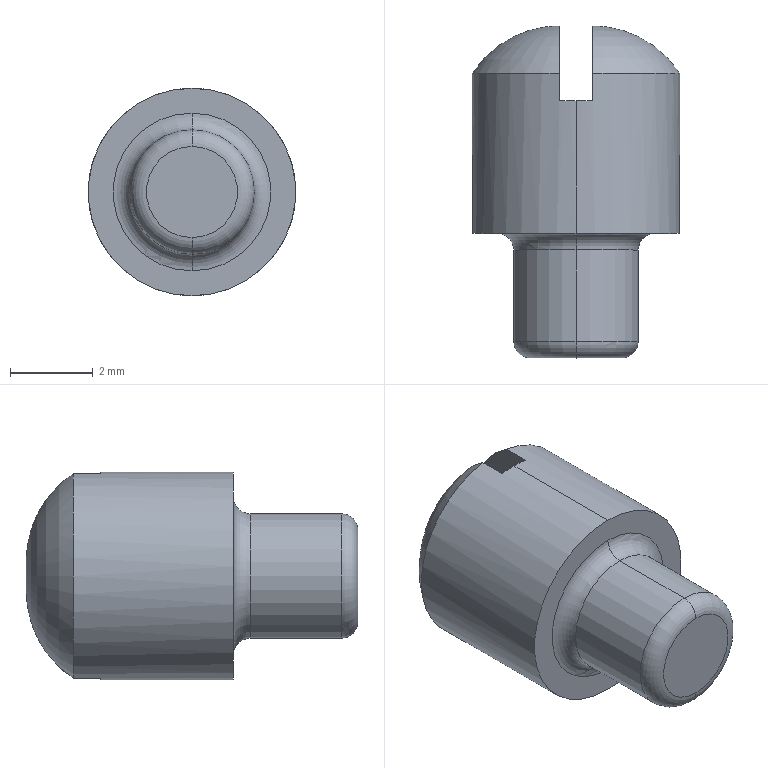Part | SolidWorks | features Fillet 2, ICE 1, Revolution 1 | 1 solid | 15 faces | box 5 x 8 x 5 mm | volume 104.473 mm3 | torus 6 | plane 5 | cylinder 4 | commonest cylinder face diameters 3 x2 5 x2
STEP:
#1=CARTESIAN_POINT('',(0.,0.4,1.5));
#2=VERTEX_POINT('',#1);
#3=CARTESIAN_POINT('',(0.,0.4,-1.5));
#4=VERTEX_POINT('',#3);
#5=CARTESIAN_POINT('',(0.,0.4,0.));
#6=DIRECTION('',(0.,1.,0.));
#7=DIRECTION('',(0.,0.,-1.));
#8=AXIS2_PLACEMENT_3D('',#5,#6,#7);
#9=CIRCLE('',#8,1.5);
#10=EDGE_CURVE('',#2,#4,#9,.T.);
#11=ORIENTED_EDGE('',*,*,#10,.F.);
#12=CARTESIAN_POINT('',(0.,0.,1.1));
#13=VERTEX_POINT('',#12);
#14=CARTESIAN_POINT('',(0.,0.4,1.1));
#15=DIRECTION('',(1.,0.,0.));
#16=DIRECTION('',(0.,0.,-1.));
#17=AXIS2_PLACEMENT_3D('',#14,#15,#16);
#18=CIRCLE('',#17,0.4);
#19=EDGE_CURVE('',#2,#13,#18,.T.);
#20=ORIENTED_EDGE('',*,*,#19,.T.);
#21=CARTESIAN_POINT('',(0.,0.,-1.1));
#22=VERTEX_POINT('',#21);
#23=CARTESIAN_POINT('',(0.,0.,0.));
#24=DIRECTION('',(0.,-1.,0.));
#25=DIRECTION('',(0.,0.,-1.));
#26=AXIS2_PLACEMENT_3D('',#23,#24,#25);
#27=CIRCLE('',#26,1.1);
#28=EDGE_CURVE('',#22,#13,#27,.T.);
#29=ORIENTED_EDGE('',*,*,#28,.F.);
#30=CARTESIAN_POINT('',(0.,0.4,-1.1));
#31=DIRECTION('',(-1.,0.,0.));
#32=DIRECTION('',(0.,0.,1.));
#33=AXIS2_PLACEMENT_3D('',#30,#31,#32);
#34=CIRCLE('',#33,0.4);
#35=EDGE_CURVE('',#4,#22,#34,.T.);
#36=ORIENTED_EDGE('',*,*,#35,.F.);
#37=EDGE_LOOP('',(#11,#20,#29,#36));
#38=FACE_OUTER_BOUND('',#37,.T.);
#39=CARTESIAN_POINT('',(0.,0.4,0.));
#40=DIRECTION('',(0.,-1.,0.));
#41=DIRECTION('',(0.,0.,-1.));
#42=AXIS2_PLACEMENT_3D('',#39,#40,#41);
#43=TOROIDAL_SURFACE('',#42,1.1,0.4);
#44=ADVANCED_FACE('',(#38),#43,.T.);
#45=CARTESIAN_POINT('',(0.,2.6,1.5));
#46=VERTEX_POINT('',#45);
#47=CARTESIAN_POINT('',(0.,2.6,-1.5));
#48=VERTEX_POINT('',#47);
#49=CARTESIAN_POINT('',(0.,2.6,0.));
#50=DIRECTION('',(0.,-1.,0.));
#51=DIRECTION('',(0.,0.,-1.));
#52=AXIS2_PLACEMENT_3D('',#49,#50,#51);
#53=CIRCLE('',#52,1.5);
#54=EDGE_CURVE('',#46,#48,#53,.T.);
#55=ORIENTED_EDGE('',*,*,#54,.F.);
#56=CARTESIAN_POINT('',(0.,3.,1.9));
#57=VERTEX_POINT('',#56);
#58=CARTESIAN_POINT('',(0.,2.6,1.9));
#59=DIRECTION('',(1.,0.,0.));
#60=DIRECTION('',(0.,0.,-1.));
#61=AXIS2_PLACEMENT_3D('',#58,#59,#60);
#62=CIRCLE('',#61,0.4);
#63=EDGE_CURVE('',#46,#57,#62,.T.);
#64=ORIENTED_EDGE('',*,*,#63,.T.);
#65=CARTESIAN_POINT('',(0.,3.,-1.9));
#66=VERTEX_POINT('',#65);
#67=CARTESIAN_POINT('',(0.,3.,0.));
#68=DIRECTION('',(0.,1.,0.));
#69=DIRECTION('',(0.,0.,-1.));
#70=AXIS2_PLACEMENT_3D('',#67,#68,#69);
#71=CIRCLE('',#70,1.9);
#72=EDGE_CURVE('',#66,#57,#71,.T.);
#73=ORIENTED_EDGE('',*,*,#72,.F.);
#74=CARTESIAN_POINT('',(0.,2.6,-1.9));
#75=DIRECTION('',(-1.,0.,0.));
#76=DIRECTION('',(0.,0.,1.));
#77=AXIS2_PLACEMENT_3D('',#74,#75,#76);
#78=CIRCLE('',#77,0.4);
#79=EDGE_CURVE('',#48,#66,#78,.T.);
#80=ORIENTED_EDGE('',*,*,#79,.F.);
#81=EDGE_LOOP('',(#55,#64,#73,#80));
#82=FACE_OUTER_BOUND('',#81,.T.);
#83=CARTESIAN_POINT('',(0.,2.6,0.));
#84=DIRECTION('',(0.,-1.,0.));
#85=DIRECTION('',(0.,0.,-1.));
#86=AXIS2_PLACEMENT_3D('',#83,#84,#85);
#87=TOROIDAL_SURFACE('',#86,1.9,0.4);
#88=ADVANCED_FACE('',(#82),#87,.F.);
#89=ORIENTED_EDGE('',*,*,#10,.T.);
#90=CARTESIAN_POINT('',(0.,5.056,-1.5));
#91=DIRECTION('',(0.,1.,0.));
#92=VECTOR('',#91,1000.);
#93=LINE('',#90,#92);
#94=EDGE_CURVE('',#4,#48,#93,.T.);
#95=ORIENTED_EDGE('',*,*,#94,.T.);
#96=CARTESIAN_POINT('',(0.,2.6,0.));
#97=DIRECTION('',(0.,-1.,0.));
#98=DIRECTION('',(0.,0.,-1.));
#99=AXIS2_PLACEMENT_3D('',#96,#97,#98);
#100=CIRCLE('',#99,1.5);
#101=EDGE_CURVE('',#48,#46,#100,.T.);
#102=ORIENTED_EDGE('',*,*,#101,.T.);
#103=CARTESIAN_POINT('',(0.,5.056,1.5));
#104=DIRECTION('',(0.,1.,0.));
#105=VECTOR('',#104,1000.);
#106=LINE('',#103,#105);
#107=EDGE_CURVE('',#2,#46,#106,.T.);
#108=ORIENTED_EDGE('',*,*,#107,.F.);
#109=EDGE_LOOP('',(#89,#95,#102,#108));
#110=FACE_OUTER_BOUND('',#109,.T.);
#111=CARTESIAN_POINT('',(0.,5.056,0.));
#112=DIRECTION('',(0.,1.,0.));
#113=DIRECTION('',(0.,0.,1.));
#114=AXIS2_PLACEMENT_3D('',#111,#112,#113);
#115=CYLINDRICAL_SURFACE('',#114,1.5);
#116=ADVANCED_FACE('',(#110),#115,.T.);
#117=CARTESIAN_POINT('',(0.,3.,2.5));
#118=VERTEX_POINT('',#117);
#119=CARTESIAN_POINT('',(0.,3.,-2.5));
#120=VERTEX_POINT('',#119);
#121=CARTESIAN_POINT('',(0.,3.,0.));
#122=DIRECTION('',(0.,1.,0.));
#123=DIRECTION('',(0.,0.,1.));
#124=AXIS2_PLACEMENT_3D('',#121,#122,#123);
#125=CIRCLE('',#124,2.5);
#126=EDGE_CURVE('',#118,#120,#125,.T.);
#127=ORIENTED_EDGE('',*,*,#126,.T.);
#128=CARTESIAN_POINT('',(0.,6.2,-2.5));
#129=VERTEX_POINT('',#128);
#130=CARTESIAN_POINT('',(0.,5.056,-2.5));
#131=DIRECTION('',(0.,1.,0.));
#132=VECTOR('',#131,1000.);
#133=LINE('',#130,#132);
#134=EDGE_CURVE('',#120,#129,#133,.T.);
#135=ORIENTED_EDGE('',*,*,#134,.T.);
#136=CARTESIAN_POINT('',(0.4,6.2,-2.468));
#137=VERTEX_POINT('',#136);
#138=CARTESIAN_POINT('',(0.,6.2,0.));
#139=DIRECTION('',(0.,1.,0.));
#140=DIRECTION('',(0.,0.,-1.));
#141=AXIS2_PLACEMENT_3D('',#138,#139,#140);
#142=CIRCLE('',#141,2.5);
#143=EDGE_CURVE('',#137,#129,#142,.T.);
#144=ORIENTED_EDGE('',*,*,#143,.F.);
#145=CARTESIAN_POINT('',(0.4,6.856,-2.468));
#146=VERTEX_POINT('',#145);
#147=CARTESIAN_POINT('',(0.4,5.056,-2.468));
#148=DIRECTION('',(0.,-1.,0.));
#149=VECTOR('',#148,1000.);
#150=LINE('',#147,#149);
#151=EDGE_CURVE('',#146,#137,#150,.T.);
#152=ORIENTED_EDGE('',*,*,#151,.F.);
#153=CARTESIAN_POINT('',(0.4,6.856,2.468));
#154=VERTEX_POINT('',#153);
#155=CARTESIAN_POINT('',(0.,6.856,0.));
#156=DIRECTION('',(0.,1.,0.));
#157=DIRECTION('',(0.,0.,1.));
#158=AXIS2_PLACEMENT_3D('',#155,#156,#157);
#159=CIRCLE('',#158,2.5);
#160=EDGE_CURVE('',#154,#146,#159,.T.);
#161=ORIENTED_EDGE('',*,*,#160,.F.);
#162=CARTESIAN_POINT('',(0.4,6.2,2.468));
#163=VERTEX_POINT('',#162);
#164=CARTESIAN_POINT('',(0.4,5.056,2.468));
#165=DIRECTION('',(0.,1.,0.));
#166=VECTOR('',#165,1000.);
#167=LINE('',#164,#166);
#168=EDGE_CURVE('',#163,#154,#167,.T.);
#169=ORIENTED_EDGE('',*,*,#168,.F.);
#170=CARTESIAN_POINT('',(0.,6.2,2.5));
#171=VERTEX_POINT('',#170);
#172=CARTESIAN_POINT('',(0.,6.2,0.));
#173=DIRECTION('',(0.,1.,0.));
#174=DIRECTION('',(0.,0.,-1.));
#175=AXIS2_PLACEMENT_3D('',#172,#173,#174);
#176=CIRCLE('',#175,2.5);
#177=EDGE_CURVE('',#171,#163,#176,.T.);
#178=ORIENTED_EDGE('',*,*,#177,.F.);
#179=CARTESIAN_POINT('',(0.,5.056,2.5));
#180=DIRECTION('',(0.,1.,0.));
#181=VECTOR('',#180,1000.);
#182=LINE('',#179,#181);
#183=EDGE_CURVE('',#118,#171,#182,.T.);
#184=ORIENTED_EDGE('',*,*,#183,.F.);
#185=EDGE_LOOP('',(#127,#135,#144,#152,#161,#169,#178,#184));
#186=FACE_OUTER_BOUND('',#185,.T.);
#187=CARTESIAN_POINT('',(0.,5.056,0.));
#188=DIRECTION('',(0.,1.,0.));
#189=DIRECTION('',(0.,0.,1.));
#190=AXIS2_PLACEMENT_3D('',#187,#188,#189);
#191=CYLINDRICAL_SURFACE('',#190,2.5);
#192=ADVANCED_FACE('',(#186),#191,.T.);
#193=CARTESIAN_POINT('',(-0.4,6.856,-2.468));
#194=VERTEX_POINT('',#193);
#195=CARTESIAN_POINT('',(-0.4,6.856,2.468));
#196=VERTEX_POINT('',#195);
#197=CARTESIAN_POINT('',(-0.4,6.856,-2.468));
#198=CARTESIAN_POINT('',(-0.4,6.956,-2.402));
#199=CARTESIAN_POINT('',(-0.4,7.053,-2.329));
#200=CARTESIAN_POINT('',(-0.4,7.231,-2.171));
#201=CARTESIAN_POINT('',(-0.4,7.314,-2.086));
#202=CARTESIAN_POINT('',(-0.4,7.545,-1.814));
#203=CARTESIAN_POINT('',(-0.4,7.674,-1.608));
#204=CARTESIAN_POINT('',(-0.4,7.866,-1.174));
#205=CARTESIAN_POINT('',(-0.4,7.932,-0.9402));
#206=CARTESIAN_POINT('',(-0.4,8.,-0.4697));
#207=CARTESIAN_POINT('',(-0.4,8.,-0.2315));
#208=CARTESIAN_POINT('',(-0.4,8.,0.2461));
#209=CARTESIAN_POINT('',(-0.4,7.999,0.4863));
#210=CARTESIAN_POINT('',(-0.4,7.946,0.8376));
#211=CARTESIAN_POINT('',(-0.4,7.921,0.9533));
#212=CARTESIAN_POINT('',(-0.4,7.855,1.182));
#213=CARTESIAN_POINT('',(-0.4,7.813,1.295));
#214=CARTESIAN_POINT('',(-0.4,7.668,1.618));
#215=CARTESIAN_POINT('',(-0.4,7.543,1.817));
#216=CARTESIAN_POINT('',(-0.4,7.233,2.181));
#217=CARTESIAN_POINT('',(-0.4,7.055,2.338));
#218=CARTESIAN_POINT('',(-0.4,6.856,2.468));
#219=B_SPLINE_CURVE_WITH_KNOTS('',3,(#197,#198,#199,#200,#201,#202,#203,#204,#205,#206,#207,#208,#209,#210,#211,#212,#213,#214,#215,#216,#217,#218),.UNSPECIFIED.,.F.,.F.,(4,2,2,2,2,2,2,2,2,2,4),(0.01437,0.01472,0.01508,0.0158,0.01652,0.01723,0.01795,0.01831,0.01866,0.01938,0.0201),.UNSPECIFIED.);
#220=EDGE_CURVE('',#194,#196,#219,.T.);
#221=ORIENTED_EDGE('',*,*,#220,.F.);
#222=CARTESIAN_POINT('',(0.,6.856,0.));
#223=DIRECTION('',(0.,1.,0.));
#224=DIRECTION('',(0.,0.,1.));
#225=AXIS2_PLACEMENT_3D('',#222,#223,#224);
#226=CIRCLE('',#225,2.5);
#227=EDGE_CURVE('',#194,#196,#226,.T.);
#228=ORIENTED_EDGE('',*,*,#227,.T.);
#229=EDGE_LOOP('',(#221,#228));
#230=FACE_OUTER_BOUND('',#229,.T.);
#231=CARTESIAN_POINT('',(0.,5.5,0.));
#232=DIRECTION('',(0.,1.,0.));
#233=DIRECTION('',(0.,0.,1.));
#234=AXIS2_PLACEMENT_3D('',#231,#232,#233);
#235=TOROIDAL_SURFACE('',#234,0.4,2.5);
#236=ADVANCED_FACE('',(#230),#235,.T.);
#237=ORIENTED_EDGE('',*,*,#28,.T.);
#238=CARTESIAN_POINT('',(0.,0.,0.));
#239=DIRECTION('',(0.,-1.,0.));
#240=DIRECTION('',(0.,0.,-1.));
#241=AXIS2_PLACEMENT_3D('',#238,#239,#240);
#242=CIRCLE('',#241,1.1);
#243=EDGE_CURVE('',#13,#22,#242,.T.);
#244=ORIENTED_EDGE('',*,*,#243,.T.);
#245=EDGE_LOOP('',(#237,#244));
#246=FACE_OUTER_BOUND('',#245,.T.);
#247=CARTESIAN_POINT('',(0.,0.,0.));
#248=DIRECTION('',(0.,-1.,0.));
#249=DIRECTION('',(0.,0.,-1.));
#250=AXIS2_PLACEMENT_3D('',#247,#248,#249);
#251=PLANE('',#250);
#252=ADVANCED_FACE('',(#246),#251,.T.);
#253=CARTESIAN_POINT('',(0.4,6.856,2.468));
#254=CARTESIAN_POINT('',(0.4,6.956,2.402));
#255=CARTESIAN_POINT('',(0.4,7.053,2.329));
#256=CARTESIAN_POINT('',(0.4,7.231,2.171));
#257=CARTESIAN_POINT('',(0.4,7.314,2.086));
#258=CARTESIAN_POINT('',(0.4,7.545,1.814));
#259=CARTESIAN_POINT('',(0.4,7.674,1.608));
#260=CARTESIAN_POINT('',(0.4,7.866,1.174));
#261=CARTESIAN_POINT('',(0.4,7.932,0.9402));
#262=CARTESIAN_POINT('',(0.4,8.,0.4697));
#263=CARTESIAN_POINT('',(0.4,8.,0.2315));
#264=CARTESIAN_POINT('',(0.4,8.,-0.2461));
#265=CARTESIAN_POINT('',(0.4,7.999,-0.4863));
#266=CARTESIAN_POINT('',(0.4,7.946,-0.8376));
#267=CARTESIAN_POINT('',(0.4,7.921,-0.9533));
#268=CARTESIAN_POINT('',(0.4,7.855,-1.182));
#269=CARTESIAN_POINT('',(0.4,7.813,-1.295));
#270=CARTESIAN_POINT('',(0.4,7.668,-1.618));
#271=CARTESIAN_POINT('',(0.4,7.543,-1.817));
#272=CARTESIAN_POINT('',(0.4,7.233,-2.181));
#273=CARTESIAN_POINT('',(0.4,7.055,-2.338));
#274=CARTESIAN_POINT('',(0.4,6.856,-2.468));
#275=B_SPLINE_CURVE_WITH_KNOTS('',3,(#253,#254,#255,#256,#257,#258,#259,#260,#261,#262,#263,#264,#265,#266,#267,#268,#269,#270,#271,#272,#273,#274),.UNSPECIFIED.,.F.,.F.,(4,2,2,2,2,2,2,2,2,2,4),(0.01437,0.01472,0.01508,0.0158,0.01652,0.01723,0.01795,0.01831,0.01866,0.01938,0.0201),.UNSPECIFIED.);
#276=EDGE_CURVE('',#154,#146,#275,.T.);
#277=ORIENTED_EDGE('',*,*,#276,.F.);
#278=ORIENTED_EDGE('',*,*,#160,.T.);
#279=EDGE_LOOP('',(#277,#278));
#280=FACE_OUTER_BOUND('',#279,.T.);
#281=CARTESIAN_POINT('',(0.,5.5,0.));
#282=DIRECTION('',(0.,1.,0.));
#283=DIRECTION('',(0.,0.,1.));
#284=AXIS2_PLACEMENT_3D('',#281,#282,#283);
#285=TOROIDAL_SURFACE('',#284,0.4,2.5);
#286=ADVANCED_FACE('',(#280),#285,.T.);
#287=ORIENTED_EDGE('',*,*,#134,.F.);
#288=CARTESIAN_POINT('',(0.,3.,0.));
#289=DIRECTION('',(0.,1.,0.));
#290=DIRECTION('',(0.,0.,1.));
#291=AXIS2_PLACEMENT_3D('',#288,#289,#290);
#292=CIRCLE('',#291,2.5);
#293=EDGE_CURVE('',#120,#118,#292,.T.);
#294=ORIENTED_EDGE('',*,*,#293,.T.);
#295=ORIENTED_EDGE('',*,*,#183,.T.);
#296=CARTESIAN_POINT('',(-0.4,6.2,2.468));
#297=VERTEX_POINT('',#296);
#298=CARTESIAN_POINT('',(0.,6.2,0.));
#299=DIRECTION('',(0.,1.,0.));
#300=DIRECTION('',(0.,0.,-1.));
#301=AXIS2_PLACEMENT_3D('',#298,#299,#300);
#302=CIRCLE('',#301,2.5);
#303=EDGE_CURVE('',#297,#171,#302,.T.);
#304=ORIENTED_EDGE('',*,*,#303,.F.);
#305=CARTESIAN_POINT('',(-0.4,5.056,2.468));
#306=DIRECTION('',(0.,-1.,0.));
#307=VECTOR('',#306,1000.);
#308=LINE('',#305,#307);
#309=EDGE_CURVE('',#196,#297,#308,.T.);
#310=ORIENTED_EDGE('',*,*,#309,.F.);
#311=ORIENTED_EDGE('',*,*,#227,.F.);
#312=CARTESIAN_POINT('',(-0.4,6.2,-2.468));
#313=VERTEX_POINT('',#312);
#314=CARTESIAN_POINT('',(-0.4,5.056,-2.468));
#315=DIRECTION('',(0.,1.,0.));
#316=VECTOR('',#315,1000.);
#317=LINE('',#314,#316);
#318=EDGE_CURVE('',#313,#194,#317,.T.);
#319=ORIENTED_EDGE('',*,*,#318,.F.);
#320=CARTESIAN_POINT('',(0.,6.2,0.));
#321=DIRECTION('',(0.,1.,0.));
#322=DIRECTION('',(0.,0.,-1.));
#323=AXIS2_PLACEMENT_3D('',#320,#321,#322);
#324=CIRCLE('',#323,2.5);
#325=EDGE_CURVE('',#129,#313,#324,.T.);
#326=ORIENTED_EDGE('',*,*,#325,.F.);
#327=EDGE_LOOP('',(#287,#294,#295,#304,#310,#311,#319,#326));
#328=FACE_OUTER_BOUND('',#327,.T.);
#329=CARTESIAN_POINT('',(0.,5.056,0.));
#330=DIRECTION('',(0.,1.,0.));
#331=DIRECTION('',(0.,0.,1.));
#332=AXIS2_PLACEMENT_3D('',#329,#330,#331);
#333=CYLINDRICAL_SURFACE('',#332,2.5);
#334=ADVANCED_FACE('',(#328),#333,.T.);
#335=ORIENTED_EDGE('',*,*,#72,.T.);
#336=CARTESIAN_POINT('',(0.,3.,0.));
#337=DIRECTION('',(0.,1.,0.));
#338=DIRECTION('',(0.,0.,-1.));
#339=AXIS2_PLACEMENT_3D('',#336,#337,#338);
#340=CIRCLE('',#339,1.9);
#341=EDGE_CURVE('',#57,#66,#340,.T.);
#342=ORIENTED_EDGE('',*,*,#341,.T.);
#343=EDGE_LOOP('',(#335,#342));
#344=FACE_BOUND('',#343,.T.);
#345=ORIENTED_EDGE('',*,*,#126,.F.);
#346=ORIENTED_EDGE('',*,*,#293,.F.);
#347=EDGE_LOOP('',(#345,#346));
#348=FACE_OUTER_BOUND('',#347,.T.);
#349=CARTESIAN_POINT('',(-1.5,3.,0.));
#350=DIRECTION('',(0.,-1.,0.));
#351=DIRECTION('',(0.,0.,-1.));
#352=AXIS2_PLACEMENT_3D('',#349,#350,#351);
#353=PLANE('',#352);
#354=ADVANCED_FACE('',(#344,#348),#353,.T.);
#355=ORIENTED_EDGE('',*,*,#94,.F.);
#356=CARTESIAN_POINT('',(0.,0.4,0.));
#357=DIRECTION('',(0.,1.,0.));
#358=DIRECTION('',(0.,0.,-1.));
#359=AXIS2_PLACEMENT_3D('',#356,#357,#358);
#360=CIRCLE('',#359,1.5);
#361=EDGE_CURVE('',#4,#2,#360,.T.);
#362=ORIENTED_EDGE('',*,*,#361,.T.);
#363=ORIENTED_EDGE('',*,*,#107,.T.);
#364=ORIENTED_EDGE('',*,*,#54,.T.);
#365=EDGE_LOOP('',(#355,#362,#363,#364));
#366=FACE_OUTER_BOUND('',#365,.T.);
#367=CARTESIAN_POINT('',(0.,5.056,0.));
#368=DIRECTION('',(0.,1.,0.));
#369=DIRECTION('',(0.,0.,1.));
#370=AXIS2_PLACEMENT_3D('',#367,#368,#369);
#371=CYLINDRICAL_SURFACE('',#370,1.5);
#372=ADVANCED_FACE('',(#366),#371,.T.);
#373=ORIENTED_EDGE('',*,*,#63,.F.);
#374=ORIENTED_EDGE('',*,*,#101,.F.);
#375=ORIENTED_EDGE('',*,*,#79,.T.);
#376=ORIENTED_EDGE('',*,*,#341,.F.);
#377=EDGE_LOOP('',(#373,#374,#375,#376));
#378=FACE_OUTER_BOUND('',#377,.T.);
#379=CARTESIAN_POINT('',(0.,2.6,0.));
#380=DIRECTION('',(0.,-1.,0.));
#381=DIRECTION('',(0.,0.,-1.));
#382=AXIS2_PLACEMENT_3D('',#379,#380,#381);
#383=TOROIDAL_SURFACE('',#382,1.9,0.4);
#384=ADVANCED_FACE('',(#378),#383,.F.);
#385=ORIENTED_EDGE('',*,*,#19,.F.);
#386=ORIENTED_EDGE('',*,*,#361,.F.);
#387=ORIENTED_EDGE('',*,*,#35,.T.);
#388=ORIENTED_EDGE('',*,*,#243,.F.);
#389=EDGE_LOOP('',(#385,#386,#387,#388));
#390=FACE_OUTER_BOUND('',#389,.T.);
#391=CARTESIAN_POINT('',(0.,0.4,0.));
#392=DIRECTION('',(0.,-1.,0.));
#393=DIRECTION('',(0.,0.,-1.));
#394=AXIS2_PLACEMENT_3D('',#391,#392,#393);
#395=TOROIDAL_SURFACE('',#394,1.1,0.4);
#396=ADVANCED_FACE('',(#390),#395,.T.);
#397=ORIENTED_EDGE('',*,*,#309,.T.);
#398=CARTESIAN_POINT('',(-0.4,6.2,-5.));
#399=DIRECTION('',(0.,0.,1.));
#400=VECTOR('',#399,1000.);
#401=LINE('',#398,#400);
#402=EDGE_CURVE('',#313,#297,#401,.T.);
#403=ORIENTED_EDGE('',*,*,#402,.F.);
#404=ORIENTED_EDGE('',*,*,#318,.T.);
#405=ORIENTED_EDGE('',*,*,#220,.T.);
#406=EDGE_LOOP('',(#397,#403,#404,#405));
#407=FACE_OUTER_BOUND('',#406,.T.);
#408=CARTESIAN_POINT('',(-0.4,8.,-5.));
#409=DIRECTION('',(-1.,0.,0.));
#410=DIRECTION('',(0.,-1.,0.));
#411=AXIS2_PLACEMENT_3D('',#408,#409,#410);
#412=PLANE('',#411);
#413=ADVANCED_FACE('',(#407),#412,.F.);
#414=ORIENTED_EDGE('',*,*,#151,.T.);
#415=CARTESIAN_POINT('',(0.4,6.2,-5.));
#416=DIRECTION('',(0.,0.,1.));
#417=VECTOR('',#416,1000.);
#418=LINE('',#415,#417);
#419=EDGE_CURVE('',#137,#163,#418,.T.);
#420=ORIENTED_EDGE('',*,*,#419,.T.);
#421=ORIENTED_EDGE('',*,*,#168,.T.);
#422=ORIENTED_EDGE('',*,*,#276,.T.);
#423=EDGE_LOOP('',(#414,#420,#421,#422));
#424=FACE_OUTER_BOUND('',#423,.T.);
#425=CARTESIAN_POINT('',(0.4,8.,-5.));
#426=DIRECTION('',(1.,0.,0.));
#427=DIRECTION('',(0.,1.,0.));
#428=AXIS2_PLACEMENT_3D('',#425,#426,#427);
#429=PLANE('',#428);
#430=ADVANCED_FACE('',(#424),#429,.F.);
#431=ORIENTED_EDGE('',*,*,#303,.T.);
#432=ORIENTED_EDGE('',*,*,#177,.T.);
#433=ORIENTED_EDGE('',*,*,#419,.F.);
#434=ORIENTED_EDGE('',*,*,#143,.T.);
#435=ORIENTED_EDGE('',*,*,#325,.T.);
#436=ORIENTED_EDGE('',*,*,#402,.T.);
#437=EDGE_LOOP('',(#431,#432,#433,#434,#435,#436));
#438=FACE_OUTER_BOUND('',#437,.T.);
#439=CARTESIAN_POINT('',(-0.4,6.2,-5.));
#440=DIRECTION('',(0.,-1.,0.));
#441=DIRECTION('',(0.,0.,-1.));
#442=AXIS2_PLACEMENT_3D('',#439,#440,#441);
#443=PLANE('',#442);
#444=ADVANCED_FACE('',(#438),#443,.F.);
#445=CLOSED_SHELL('',(#44,#88,#116,#192,#236,#252,#286,#334,#354,#372,#384,#396,#413,#430,#444));
#446=MANIFOLD_SOLID_BREP('',#445);
#447=CARTESIAN_POINT('',(0.,0.,0.));
#448=DIRECTION('',(0.,0.,1.));
#449=DIRECTION('',(1.,0.,0.));
#450=AXIS2_PLACEMENT_3D('',#447,#448,#449);
#451=(LENGTH_UNIT()NAMED_UNIT(*)SI_UNIT(.MILLI.,.METRE.));
#452=UNCERTAINTY_MEASURE_WITH_UNIT(LENGTH_MEASURE(0.00001),#451,'','');
#453=(NAMED_UNIT(*)PLANE_ANGLE_UNIT()SI_UNIT($,.RADIAN.));
#454=(NAMED_UNIT(*)SI_UNIT($,.STERADIAN.)SOLID_ANGLE_UNIT());
#455=(GEOMETRIC_REPRESENTATION_CONTEXT(3)GLOBAL_UNCERTAINTY_ASSIGNED_CONTEXT((#452))GLOBAL_UNIT_ASSIGNED_CONTEXT((#451,#453,#454))REPRESENTATION_CONTEXT('',''));
#456=ADVANCED_BREP_SHAPE_REPRESENTATION('',(#446,#450),#455);